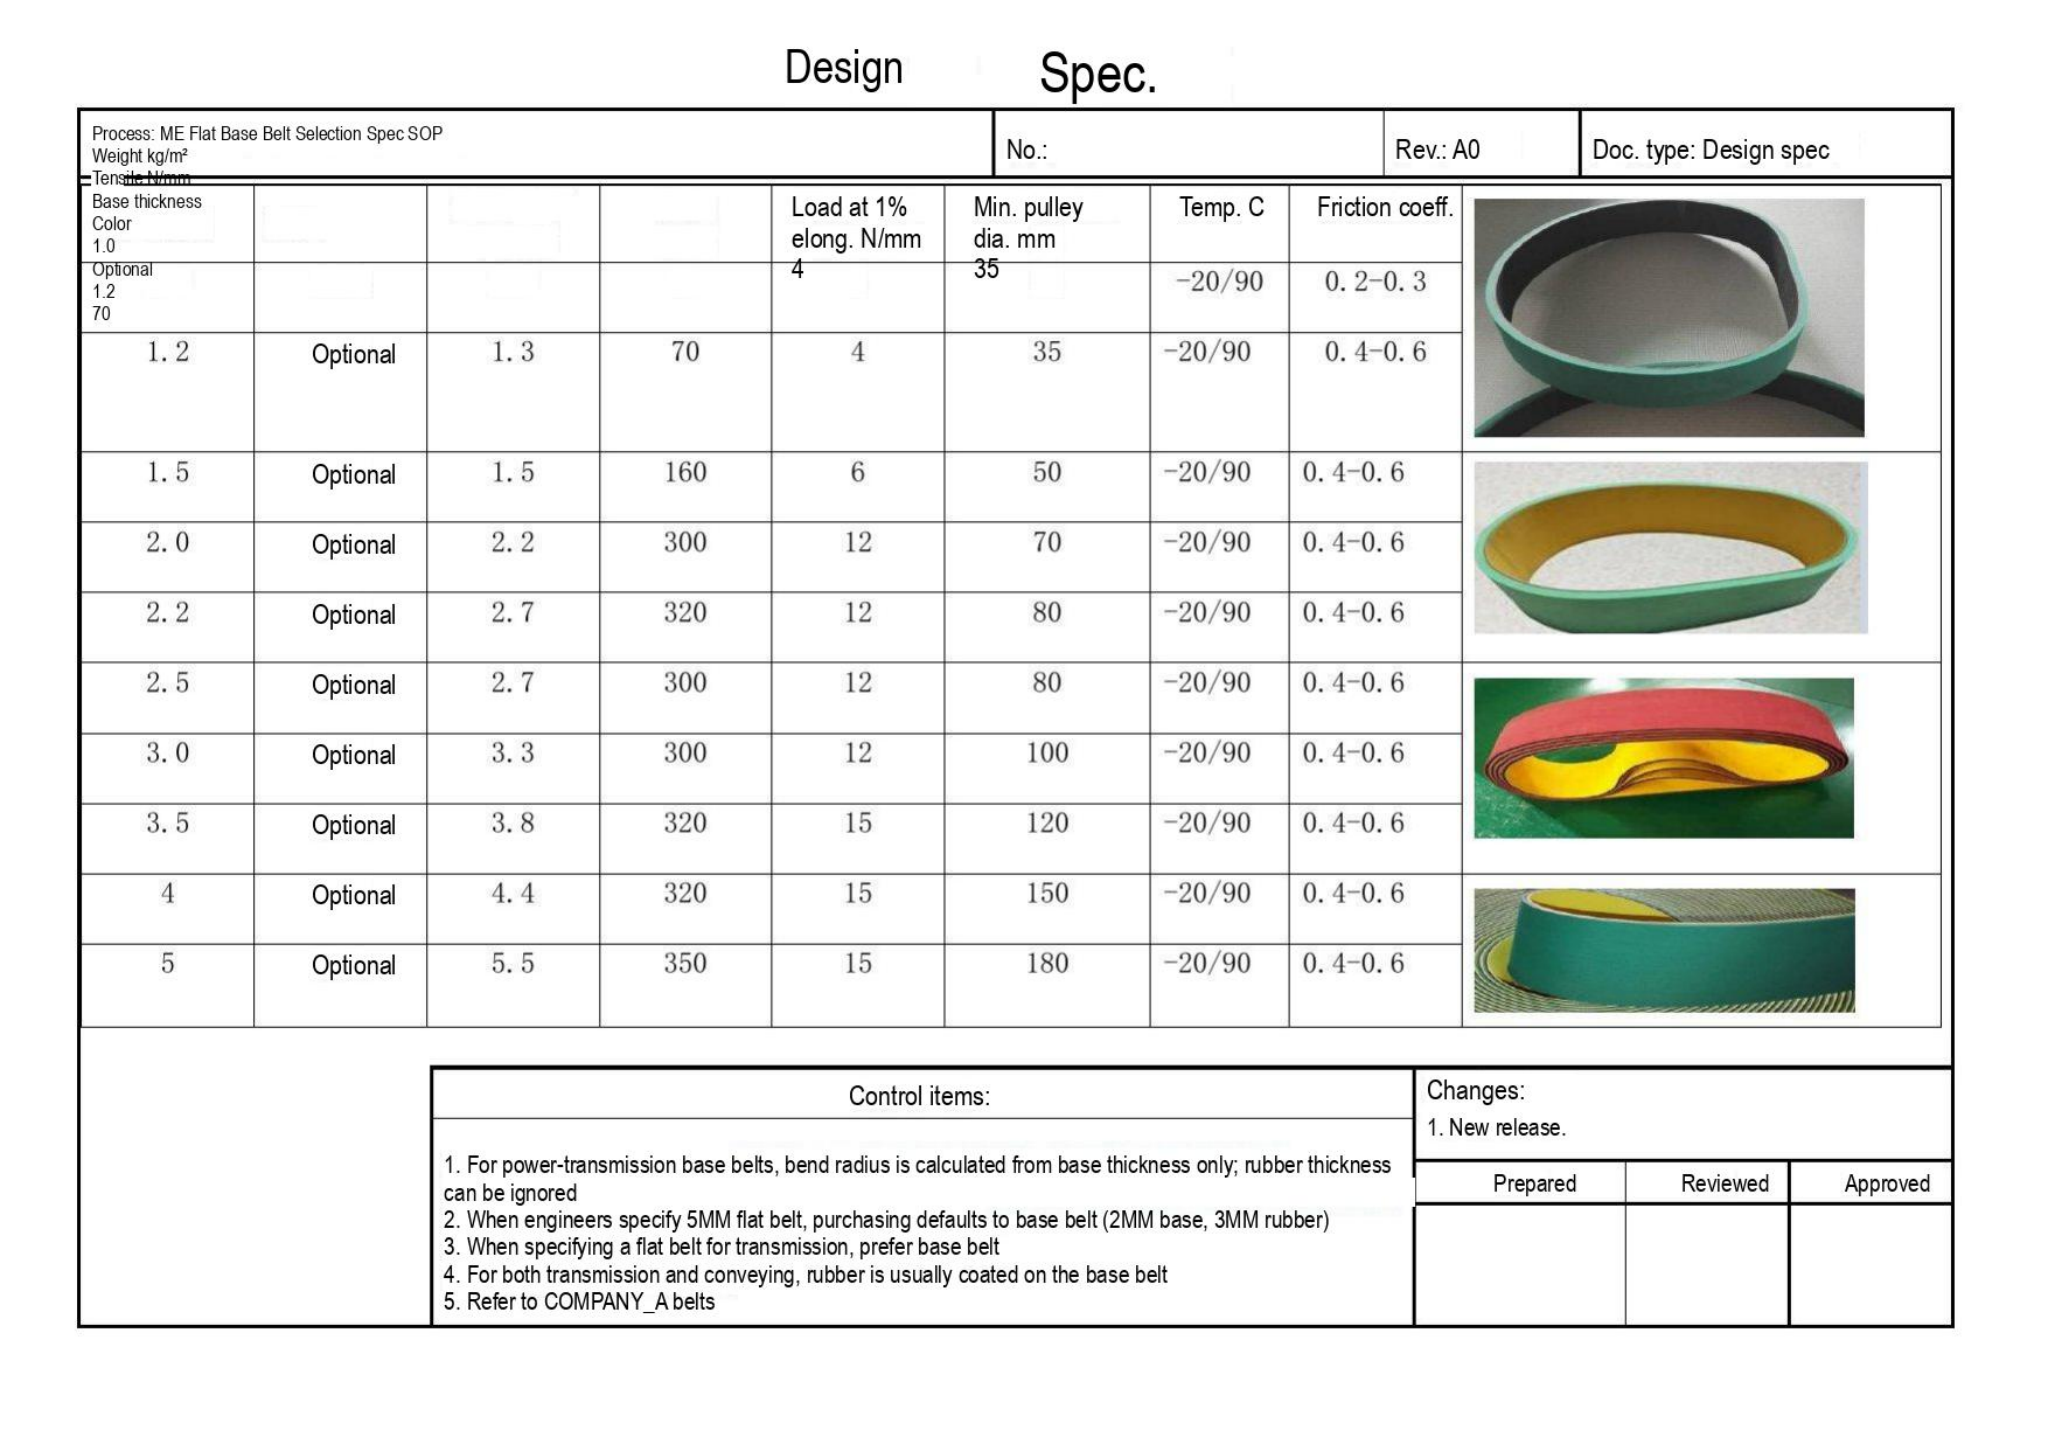Design Spec.

| Process: ME Flat Base Belt Selection Spec SOP<br>Weight kg/m²<br>Tensile N/mm | No.: | Rev.: A0 | Doc. type: Design spec |
|---|---|---|---|

| Base thickness<br>Color<br>1.0 | | | | Load at 1% elong. N/mm | Min. pulley dia. mm | Temp. C | Friction coeff. |
|---|---|---|---|---|---|---|---|
| Optional<br>1.2<br>70 | | | | 4 | 35 | -20/90 | 0. 2-0. 3 |
| 1. 2 | Optional | 1. 3 | 70 | 4 | 35 | -20/90 | 0. 4-0. 6 |
| 1. 5 | Optional | 1. 5 | 160 | 6 | 50 | -20/90 | 0. 4-0. 6 |
| 2. 0 | Optional | 2. 2 | 300 | 12 | 70 | -20/90 | 0. 4-0. 6 |
| 2. 2 | Optional | 2. 7 | 320 | 12 | 80 | -20/90 | 0. 4-0. 6 |
| 2. 5 | Optional | 2. 7 | 300 | 12 | 80 | -20/90 | 0. 4-0. 6 |
| 3. 0 | Optional | 3. 3 | 300 | 12 | 100 | -20/90 | 0. 4-0. 6 |
| 3. 5 | Optional | 3. 8 | 320 | 15 | 120 | -20/90 | 0. 4-0. 6 |
| 4 | Optional | 4. 4 | 320 | 15 | 150 | -20/90 | 0. 4-0. 6 |
| 5 | Optional | 5. 5 | 350 | 15 | 180 | -20/90 | 0. 4-0. 6 |

Control items:

1. For power-transmission base belts, bend radius is calculated from base thickness only; rubber thickness can be ignored
2. When engineers specify 5MM flat belt, purchasing defaults to base belt (2MM base, 3MM rubber)
3. When specifying a flat belt for transmission, prefer base belt
4. For both transmission and conveying, rubber is usually coated on the base belt
5. Refer to COMPANY_A belts

Changes:
1. New release.

| Prepared | Reviewed | Approved |
|---|---|---|
| | | |